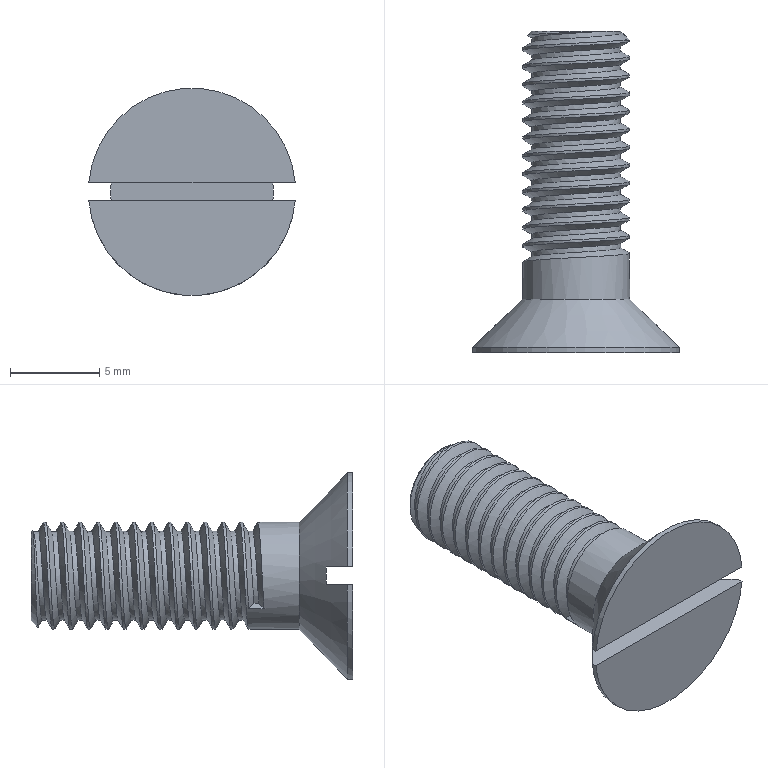Part | NX | features DATUM_CSYS 3, SKETCH 2, CHAMFER 1, CYLINDER 1, EXTRUDE 1, SWP104 1, THREADS 1 | 1 solid | 27 faces | box 11.557 x 18 x 11.6 mm | volume 532.719 mm3 | cylinder 15 | plane 8 | cone 2 | spline 2 | commonest cylinder face diameters 6 x12 11.6 x2 5 x1